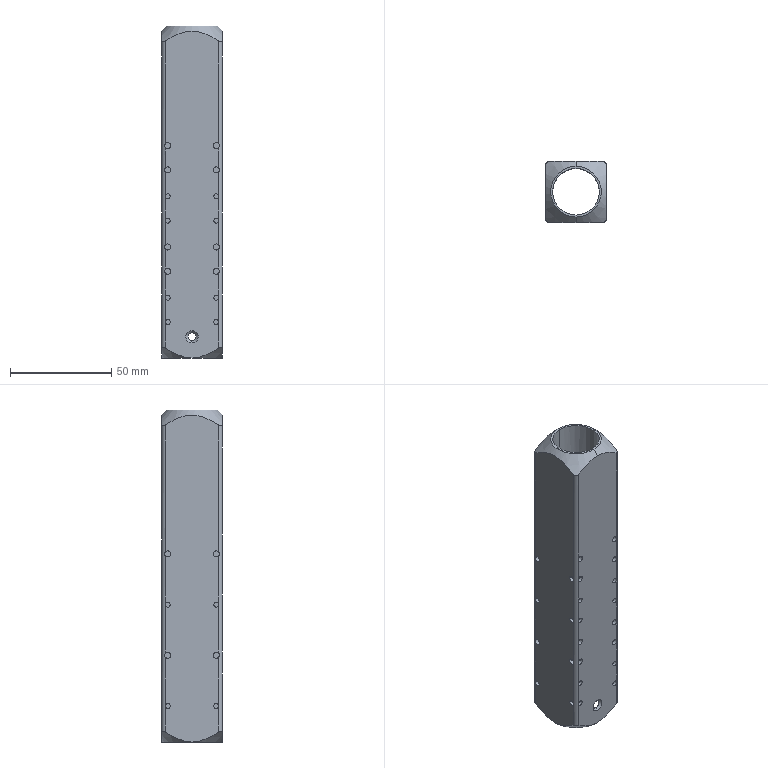Part | STEP file | ASND-0110-4216100000 | 1 solid | 204 faces | box 30 x 30 x 163.75 mm | volume 53858 mm3 | cylinder 139 | plane 49 | cone 12 | torus 4 | commonest cylinder face diameters 2.5 x52 3 x51 2.05 x18 4 x8 5 x4 23 x2